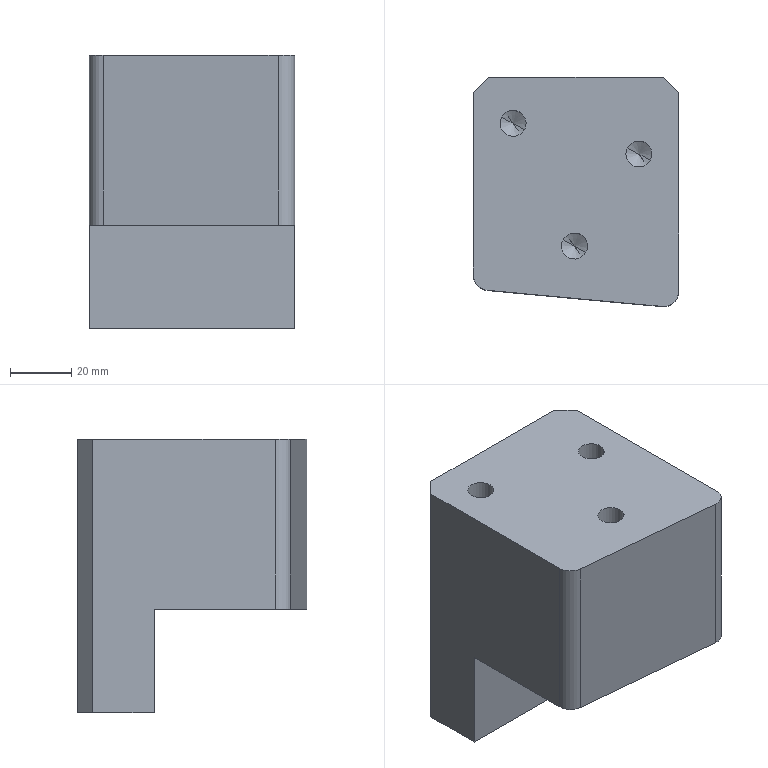Part | CATIA | 1 solid | 40 faces | box 67 x 74.702 x 89 mm | volume 308137 mm3 | cylinder 16 | cone 14 | plane 10 | commonest cylinder face diameters 8.5 x12 10 x4
STEP:
#1=CARTESIAN_POINT('',(81.,85.,84.));
#2=VERTEX_POINT('',#1);
#3=CARTESIAN_POINT('',(86.,90.,84.));
#4=VERTEX_POINT('',#3);
#5=CARTESIAN_POINT('',(83.5,87.5,84.));
#6=DIRECTION('',(-0.7071,-0.7071,0.));
#7=VECTOR('',#6,1.);
#8=LINE('',#5,#7);
#9=EDGE_CURVE('',#2,#4,#8,.F.);
#10=ORIENTED_EDGE('',*,*,#9,.T.);
#11=CARTESIAN_POINT('',(86.,90.,-5.));
#12=VERTEX_POINT('',#11);
#13=CARTESIAN_POINT('',(86.,90.,39.5));
#14=DIRECTION('',(0.,0.,-1.));
#15=VECTOR('',#14,1.);
#16=LINE('',#13,#15);
#17=EDGE_CURVE('',#12,#4,#16,.F.);
#18=ORIENTED_EDGE('',*,*,#17,.F.);
#19=CARTESIAN_POINT('',(81.,85.,-5.));
#20=VERTEX_POINT('',#19);
#21=CARTESIAN_POINT('',(83.5,87.5,-5.));
#22=DIRECTION('',(-0.7071,-0.7071,0.));
#23=VECTOR('',#22,1.);
#24=LINE('',#21,#23);
#25=EDGE_CURVE('',#12,#20,#24,.T.);
#26=ORIENTED_EDGE('',*,*,#25,.T.);
#27=CARTESIAN_POINT('',(81.,85.,39.5));
#28=DIRECTION('',(0.,0.,-1.));
#29=VECTOR('',#28,1.);
#30=LINE('',#27,#29);
#31=EDGE_CURVE('',#20,#2,#30,.F.);
#32=ORIENTED_EDGE('',*,*,#31,.T.);
#33=EDGE_LOOP('',(#10,#18,#26,#32));
#34=FACE_OUTER_BOUND('',#33,.T.);
#35=CARTESIAN_POINT('',(86.,90.,101.8));
#36=DIRECTION('',(-0.7071,0.7071,0.));
#37=DIRECTION('',(0.,0.,-1.));
#38=AXIS2_PLACEMENT_3D('',#35,#36,#37);
#39=PLANE('',#38);
#40=ADVANCED_FACE('',(#34),#39,.T.);
#41=CARTESIAN_POINT('',(143.,90.,-5.));
#42=VERTEX_POINT('',#41);
#43=CARTESIAN_POINT('',(143.,90.,84.));
#44=VERTEX_POINT('',#43);
#45=CARTESIAN_POINT('',(143.,90.,39.5));
#46=DIRECTION('',(0.,0.,1.));
#47=VECTOR('',#46,1.);
#48=LINE('',#45,#47);
#49=EDGE_CURVE('',#42,#44,#48,.T.);
#50=ORIENTED_EDGE('',*,*,#49,.F.);
#51=CARTESIAN_POINT('',(114.5,90.,-5.));
#52=DIRECTION('',(1.,0.,0.));
#53=VECTOR('',#52,1.);
#54=LINE('',#51,#53);
#55=EDGE_CURVE('',#12,#42,#54,.T.);
#56=ORIENTED_EDGE('',*,*,#55,.F.);
#57=ORIENTED_EDGE('',*,*,#17,.T.);
#58=CARTESIAN_POINT('',(114.5,90.,84.));
#59=DIRECTION('',(1.,0.,0.));
#60=VECTOR('',#59,1.);
#61=LINE('',#58,#60);
#62=EDGE_CURVE('',#4,#44,#61,.T.);
#63=ORIENTED_EDGE('',*,*,#62,.T.);
#64=EDGE_LOOP('',(#50,#56,#57,#63));
#65=FACE_OUTER_BOUND('',#64,.T.);
#66=CARTESIAN_POINT('',(81.,90.,0.));
#67=DIRECTION('',(0.,-1.,0.));
#68=DIRECTION('',(1.,0.,0.));
#69=AXIS2_PLACEMENT_3D('',#66,#67,#68);
#70=PLANE('',#69);
#71=ADVANCED_FACE('',(#65),#70,.F.);
#72=CARTESIAN_POINT('',(148.,85.,84.));
#73=VERTEX_POINT('',#72);
#74=CARTESIAN_POINT('',(145.5,87.5,84.));
#75=DIRECTION('',(0.7071,-0.7071,0.));
#76=VECTOR('',#75,1.);
#77=LINE('',#74,#76);
#78=EDGE_CURVE('',#44,#73,#77,.T.);
#79=ORIENTED_EDGE('',*,*,#78,.T.);
#80=CARTESIAN_POINT('',(148.,85.,-5.));
#81=VERTEX_POINT('',#80);
#82=CARTESIAN_POINT('',(148.,85.,39.5));
#83=DIRECTION('',(0.,0.,1.));
#84=VECTOR('',#83,1.);
#85=LINE('',#82,#84);
#86=EDGE_CURVE('',#81,#73,#85,.T.);
#87=ORIENTED_EDGE('',*,*,#86,.F.);
#88=CARTESIAN_POINT('',(145.5,87.5,-5.));
#89=DIRECTION('',(0.7071,-0.7071,0.));
#90=VECTOR('',#89,1.);
#91=LINE('',#88,#90);
#92=EDGE_CURVE('',#81,#42,#91,.F.);
#93=ORIENTED_EDGE('',*,*,#92,.T.);
#94=ORIENTED_EDGE('',*,*,#49,.T.);
#95=EDGE_LOOP('',(#79,#87,#93,#94));
#96=FACE_OUTER_BOUND('',#95,.T.);
#97=CARTESIAN_POINT('',(143.,90.,-22.8));
#98=DIRECTION('',(0.7071,0.7071,0.));
#99=DIRECTION('',(0.,0.,1.));
#100=AXIS2_PLACEMENT_3D('',#97,#98,#99);
#101=PLANE('',#100);
#102=ADVANCED_FACE('',(#96),#101,.T.);
#103=CARTESIAN_POINT('',(114.,35.,51.546));
#104=VERTEX_POINT('',#103);
#105=CARTESIAN_POINT('',(110.27,37.038,54.));
#106=VERTEX_POINT('',#105);
#107=CARTESIAN_POINT('',(112.135,36.019,52.773));
#108=DIRECTION('',(-0.76,0.4152,0.5));
#109=VECTOR('',#108,1.);
#110=LINE('',#107,#109);
#111=EDGE_CURVE('',#104,#106,#110,.T.);
#112=ORIENTED_EDGE('',*,*,#111,.T.);
#113=CARTESIAN_POINT('',(117.73,32.962,54.));
#114=VERTEX_POINT('',#113);
#115=CARTESIAN_POINT('',(114.,35.,54.));
#116=DIRECTION('',(0.,0.,1.));
#117=AXIS2_PLACEMENT_3D('',#115,#116,$);
#118=CIRCLE('',#117,4.25);
#119=EDGE_CURVE('',#114,#106,#118,.F.);
#120=ORIENTED_EDGE('',*,*,#119,.F.);
#121=CARTESIAN_POINT('',(115.865,33.981,52.773));
#122=DIRECTION('',(0.76,-0.4152,0.5));
#123=VECTOR('',#122,1.);
#124=LINE('',#121,#123);
#125=EDGE_CURVE('',#104,#114,#124,.T.);
#126=ORIENTED_EDGE('',*,*,#125,.F.);
#127=EDGE_LOOP('',(#112,#120,#126));
#128=FACE_OUTER_BOUND('',#127,.T.);
#129=CARTESIAN_POINT('',(114.,35.,51.546));
#130=DIRECTION('',(0.,0.,1.));
#131=DIRECTION('',(0.8776,-0.4794,0.));
#132=AXIS2_PLACEMENT_3D('',#129,#130,#131);
#133=CONICAL_SURFACE('',#132,0.,1.047);
#134=ADVANCED_FACE('',(#128),#133,.F.);
#135=ORIENTED_EDGE('',*,*,#125,.T.);
#136=CARTESIAN_POINT('',(114.,35.,54.));
#137=DIRECTION('',(0.,0.,1.));
#138=AXIS2_PLACEMENT_3D('',#136,#137,$);
#139=CIRCLE('',#138,4.25);
#140=EDGE_CURVE('',#106,#114,#139,.F.);
#141=ORIENTED_EDGE('',*,*,#140,.F.);
#142=ORIENTED_EDGE('',*,*,#111,.F.);
#143=EDGE_LOOP('',(#135,#141,#142));
#144=FACE_OUTER_BOUND('',#143,.T.);
#145=ADVANCED_FACE('',(#144),#133,.F.);
#146=CARTESIAN_POINT('',(110.27,37.038,84.));
#147=VERTEX_POINT('',#146);
#148=CARTESIAN_POINT('',(117.73,32.962,84.));
#149=VERTEX_POINT('',#148);
#150=CARTESIAN_POINT('',(114.,35.,84.));
#151=DIRECTION('',(0.,0.,-1.));
#152=AXIS2_PLACEMENT_3D('',#150,#151,$);
#153=CIRCLE('',#152,4.25);
#154=EDGE_CURVE('',#147,#149,#153,.F.);
#155=ORIENTED_EDGE('',*,*,#154,.T.);
#156=CARTESIAN_POINT('',(117.73,32.962,69.2));
#157=DIRECTION('',(0.,0.,-1.));
#158=VECTOR('',#157,1.);
#159=LINE('',#156,#158);
#160=EDGE_CURVE('',#114,#149,#159,.F.);
#161=ORIENTED_EDGE('',*,*,#160,.F.);
#162=ORIENTED_EDGE('',*,*,#119,.T.);
#163=CARTESIAN_POINT('',(110.27,37.038,69.2));
#164=DIRECTION('',(0.,0.,-1.));
#165=VECTOR('',#164,1.);
#166=LINE('',#163,#165);
#167=EDGE_CURVE('',#106,#147,#166,.F.);
#168=ORIENTED_EDGE('',*,*,#167,.T.);
#169=EDGE_LOOP('',(#155,#161,#162,#168));
#170=FACE_OUTER_BOUND('',#169,.T.);
#171=CARTESIAN_POINT('',(114.,35.,83.9));
#172=DIRECTION('',(0.,0.,-1.));
#173=DIRECTION('',(0.8776,-0.4794,0.));
#174=AXIS2_PLACEMENT_3D('',#171,#172,#173);
#175=CYLINDRICAL_SURFACE('',#174,4.25);
#176=ADVANCED_FACE('',(#170),#175,.F.);
#177=CARTESIAN_POINT('',(114.,35.,84.));
#178=DIRECTION('',(0.,0.,-1.));
#179=AXIS2_PLACEMENT_3D('',#177,#178,$);
#180=CIRCLE('',#179,4.25);
#181=EDGE_CURVE('',#149,#147,#180,.F.);
#182=ORIENTED_EDGE('',*,*,#181,.T.);
#183=ORIENTED_EDGE('',*,*,#167,.F.);
#184=ORIENTED_EDGE('',*,*,#140,.T.);
#185=ORIENTED_EDGE('',*,*,#160,.T.);
#186=EDGE_LOOP('',(#182,#183,#184,#185));
#187=FACE_OUTER_BOUND('',#186,.T.);
#188=ADVANCED_FACE('',(#187),#175,.F.);
#189=CARTESIAN_POINT('',(94.,75.,51.546));
#190=VERTEX_POINT('',#189);
#191=CARTESIAN_POINT('',(90.27,77.038,54.));
#192=VERTEX_POINT('',#191);
#193=CARTESIAN_POINT('',(92.135,76.019,52.773));
#194=DIRECTION('',(-0.76,0.4152,0.5));
#195=VECTOR('',#194,1.);
#196=LINE('',#193,#195);
#197=EDGE_CURVE('',#190,#192,#196,.T.);
#198=ORIENTED_EDGE('',*,*,#197,.T.);
#199=CARTESIAN_POINT('',(97.73,72.962,54.));
#200=VERTEX_POINT('',#199);
#201=CARTESIAN_POINT('',(94.,75.,54.));
#202=DIRECTION('',(0.,0.,1.));
#203=AXIS2_PLACEMENT_3D('',#201,#202,$);
#204=CIRCLE('',#203,4.25);
#205=EDGE_CURVE('',#200,#192,#204,.F.);
#206=ORIENTED_EDGE('',*,*,#205,.F.);
#207=CARTESIAN_POINT('',(95.865,73.981,52.773));
#208=DIRECTION('',(0.76,-0.4152,0.5));
#209=VECTOR('',#208,1.);
#210=LINE('',#207,#209);
#211=EDGE_CURVE('',#190,#200,#210,.T.);
#212=ORIENTED_EDGE('',*,*,#211,.F.);
#213=EDGE_LOOP('',(#198,#206,#212));
#214=FACE_OUTER_BOUND('',#213,.T.);
#215=CARTESIAN_POINT('',(94.,75.,51.546));
#216=DIRECTION('',(0.,0.,1.));
#217=DIRECTION('',(0.8776,-0.4794,0.));
#218=AXIS2_PLACEMENT_3D('',#215,#216,#217);
#219=CONICAL_SURFACE('',#218,0.,1.047);
#220=ADVANCED_FACE('',(#214),#219,.F.);
#221=ORIENTED_EDGE('',*,*,#211,.T.);
#222=CARTESIAN_POINT('',(94.,75.,54.));
#223=DIRECTION('',(0.,0.,1.));
#224=AXIS2_PLACEMENT_3D('',#222,#223,$);
#225=CIRCLE('',#224,4.25);
#226=EDGE_CURVE('',#192,#200,#225,.F.);
#227=ORIENTED_EDGE('',*,*,#226,.F.);
#228=ORIENTED_EDGE('',*,*,#197,.F.);
#229=EDGE_LOOP('',(#221,#227,#228));
#230=FACE_OUTER_BOUND('',#229,.T.);
#231=ADVANCED_FACE('',(#230),#219,.F.);
#232=CARTESIAN_POINT('',(90.27,77.038,84.));
#233=VERTEX_POINT('',#232);
#234=CARTESIAN_POINT('',(97.73,72.962,84.));
#235=VERTEX_POINT('',#234);
#236=CARTESIAN_POINT('',(94.,75.,84.));
#237=DIRECTION('',(0.,0.,-1.));
#238=AXIS2_PLACEMENT_3D('',#236,#237,$);
#239=CIRCLE('',#238,4.25);
#240=EDGE_CURVE('',#233,#235,#239,.F.);
#241=ORIENTED_EDGE('',*,*,#240,.T.);
#242=CARTESIAN_POINT('',(97.73,72.962,69.2));
#243=DIRECTION('',(0.,0.,-1.));
#244=VECTOR('',#243,1.);
#245=LINE('',#242,#244);
#246=EDGE_CURVE('',#200,#235,#245,.F.);
#247=ORIENTED_EDGE('',*,*,#246,.F.);
#248=ORIENTED_EDGE('',*,*,#205,.T.);
#249=CARTESIAN_POINT('',(90.27,77.038,69.2));
#250=DIRECTION('',(0.,0.,-1.));
#251=VECTOR('',#250,1.);
#252=LINE('',#249,#251);
#253=EDGE_CURVE('',#192,#233,#252,.F.);
#254=ORIENTED_EDGE('',*,*,#253,.T.);
#255=EDGE_LOOP('',(#241,#247,#248,#254));
#256=FACE_OUTER_BOUND('',#255,.T.);
#257=CARTESIAN_POINT('',(94.,75.,83.9));
#258=DIRECTION('',(0.,0.,-1.));
#259=DIRECTION('',(0.8776,-0.4794,0.));
#260=AXIS2_PLACEMENT_3D('',#257,#258,#259);
#261=CYLINDRICAL_SURFACE('',#260,4.25);
#262=ADVANCED_FACE('',(#256),#261,.F.);
#263=CARTESIAN_POINT('',(94.,75.,84.));
#264=DIRECTION('',(0.,0.,-1.));
#265=AXIS2_PLACEMENT_3D('',#263,#264,$);
#266=CIRCLE('',#265,4.25);
#267=EDGE_CURVE('',#235,#233,#266,.F.);
#268=ORIENTED_EDGE('',*,*,#267,.T.);
#269=ORIENTED_EDGE('',*,*,#253,.F.);
#270=ORIENTED_EDGE('',*,*,#226,.T.);
#271=ORIENTED_EDGE('',*,*,#246,.T.);
#272=EDGE_LOOP('',(#268,#269,#270,#271));
#273=FACE_OUTER_BOUND('',#272,.T.);
#274=ADVANCED_FACE('',(#273),#261,.F.);
#275=CARTESIAN_POINT('',(135.,65.,51.546));
#276=VERTEX_POINT('',#275);
#277=CARTESIAN_POINT('',(131.27,67.038,54.));
#278=VERTEX_POINT('',#277);
#279=CARTESIAN_POINT('',(133.135,66.019,52.773));
#280=DIRECTION('',(-0.76,0.4152,0.5));
#281=VECTOR('',#280,1.);
#282=LINE('',#279,#281);
#283=EDGE_CURVE('',#276,#278,#282,.T.);
#284=ORIENTED_EDGE('',*,*,#283,.T.);
#285=CARTESIAN_POINT('',(138.73,62.962,54.));
#286=VERTEX_POINT('',#285);
#287=CARTESIAN_POINT('',(135.,65.,54.));
#288=DIRECTION('',(0.,0.,1.));
#289=AXIS2_PLACEMENT_3D('',#287,#288,$);
#290=CIRCLE('',#289,4.25);
#291=EDGE_CURVE('',#286,#278,#290,.F.);
#292=ORIENTED_EDGE('',*,*,#291,.F.);
#293=CARTESIAN_POINT('',(136.865,63.981,52.773));
#294=DIRECTION('',(0.76,-0.4152,0.5));
#295=VECTOR('',#294,1.);
#296=LINE('',#293,#295);
#297=EDGE_CURVE('',#276,#286,#296,.T.);
#298=ORIENTED_EDGE('',*,*,#297,.F.);
#299=EDGE_LOOP('',(#284,#292,#298));
#300=FACE_OUTER_BOUND('',#299,.T.);
#301=CARTESIAN_POINT('',(135.,65.,51.546));
#302=DIRECTION('',(0.,0.,1.));
#303=DIRECTION('',(0.8776,-0.4794,0.));
#304=AXIS2_PLACEMENT_3D('',#301,#302,#303);
#305=CONICAL_SURFACE('',#304,0.,1.047);
#306=ADVANCED_FACE('',(#300),#305,.F.);
#307=ORIENTED_EDGE('',*,*,#297,.T.);
#308=CARTESIAN_POINT('',(135.,65.,54.));
#309=DIRECTION('',(0.,0.,1.));
#310=AXIS2_PLACEMENT_3D('',#308,#309,$);
#311=CIRCLE('',#310,4.25);
#312=EDGE_CURVE('',#278,#286,#311,.F.);
#313=ORIENTED_EDGE('',*,*,#312,.F.);
#314=ORIENTED_EDGE('',*,*,#283,.F.);
#315=EDGE_LOOP('',(#307,#313,#314));
#316=FACE_OUTER_BOUND('',#315,.T.);
#317=ADVANCED_FACE('',(#316),#305,.F.);
#318=CARTESIAN_POINT('',(131.27,67.038,84.));
#319=VERTEX_POINT('',#318);
#320=CARTESIAN_POINT('',(138.73,62.962,84.));
#321=VERTEX_POINT('',#320);
#322=CARTESIAN_POINT('',(135.,65.,84.));
#323=DIRECTION('',(0.,0.,-1.));
#324=AXIS2_PLACEMENT_3D('',#322,#323,$);
#325=CIRCLE('',#324,4.25);
#326=EDGE_CURVE('',#319,#321,#325,.F.);
#327=ORIENTED_EDGE('',*,*,#326,.T.);
#328=CARTESIAN_POINT('',(138.73,62.962,69.2));
#329=DIRECTION('',(0.,0.,-1.));
#330=VECTOR('',#329,1.);
#331=LINE('',#328,#330);
#332=EDGE_CURVE('',#286,#321,#331,.F.);
#333=ORIENTED_EDGE('',*,*,#332,.F.);
#334=ORIENTED_EDGE('',*,*,#291,.T.);
#335=CARTESIAN_POINT('',(131.27,67.038,69.2));
#336=DIRECTION('',(0.,0.,-1.));
#337=VECTOR('',#336,1.);
#338=LINE('',#335,#337);
#339=EDGE_CURVE('',#278,#319,#338,.F.);
#340=ORIENTED_EDGE('',*,*,#339,.T.);
#341=EDGE_LOOP('',(#327,#333,#334,#340));
#342=FACE_OUTER_BOUND('',#341,.T.);
#343=CARTESIAN_POINT('',(135.,65.,83.9));
#344=DIRECTION('',(0.,0.,-1.));
#345=DIRECTION('',(0.8776,-0.4794,0.));
#346=AXIS2_PLACEMENT_3D('',#343,#344,#345);
#347=CYLINDRICAL_SURFACE('',#346,4.25);
#348=ADVANCED_FACE('',(#342),#347,.F.);
#349=CARTESIAN_POINT('',(135.,65.,84.));
#350=DIRECTION('',(0.,0.,-1.));
#351=AXIS2_PLACEMENT_3D('',#349,#350,$);
#352=CIRCLE('',#351,4.25);
#353=EDGE_CURVE('',#321,#319,#352,.F.);
#354=ORIENTED_EDGE('',*,*,#353,.T.);
#355=ORIENTED_EDGE('',*,*,#339,.F.);
#356=ORIENTED_EDGE('',*,*,#312,.T.);
#357=ORIENTED_EDGE('',*,*,#332,.T.);
#358=EDGE_LOOP('',(#354,#355,#356,#357));
#359=FACE_OUTER_BOUND('',#358,.T.);
#360=ADVANCED_FACE('',(#359),#347,.F.);
#361=CARTESIAN_POINT('',(94.,52.,61.454));
#362=VERTEX_POINT('',#361);
#363=CARTESIAN_POINT('',(90.27,49.962,59.));
#364=VERTEX_POINT('',#363);
#365=CARTESIAN_POINT('',(92.135,50.981,60.227));
#366=DIRECTION('',(-0.76,-0.4152,-0.5));
#367=VECTOR('',#366,1.);
#368=LINE('',#365,#367);
#369=EDGE_CURVE('',#362,#364,#368,.T.);
#370=ORIENTED_EDGE('',*,*,#369,.T.);
#371=CARTESIAN_POINT('',(97.73,54.038,59.));
#372=VERTEX_POINT('',#371);
#373=CARTESIAN_POINT('',(94.,52.,59.));
#374=DIRECTION('',(0.,0.,-1.));
#375=AXIS2_PLACEMENT_3D('',#373,#374,$);
#376=CIRCLE('',#375,4.25);
#377=EDGE_CURVE('',#372,#364,#376,.F.);
#378=ORIENTED_EDGE('',*,*,#377,.F.);
#379=CARTESIAN_POINT('',(95.865,53.019,60.227));
#380=DIRECTION('',(0.76,0.4152,-0.5));
#381=VECTOR('',#380,1.);
#382=LINE('',#379,#381);
#383=EDGE_CURVE('',#362,#372,#382,.T.);
#384=ORIENTED_EDGE('',*,*,#383,.F.);
#385=EDGE_LOOP('',(#370,#378,#384));
#386=FACE_OUTER_BOUND('',#385,.T.);
#387=CARTESIAN_POINT('',(94.,52.,61.454));
#388=DIRECTION('',(0.,0.,-1.));
#389=DIRECTION('',(0.8776,0.4794,0.));
#390=AXIS2_PLACEMENT_3D('',#387,#388,#389);
#391=CONICAL_SURFACE('',#390,0.,1.047);
#392=ADVANCED_FACE('',(#386),#391,.F.);
#393=ORIENTED_EDGE('',*,*,#383,.T.);
#394=CARTESIAN_POINT('',(94.,52.,59.));
#395=DIRECTION('',(0.,0.,-1.));
#396=AXIS2_PLACEMENT_3D('',#394,#395,$);
#397=CIRCLE('',#396,4.25);
#398=EDGE_CURVE('',#364,#372,#397,.F.);
#399=ORIENTED_EDGE('',*,*,#398,.F.);
#400=ORIENTED_EDGE('',*,*,#369,.F.);
#401=EDGE_LOOP('',(#393,#399,#400));
#402=FACE_OUTER_BOUND('',#401,.T.);
#403=ADVANCED_FACE('',(#402),#391,.F.);
#404=CARTESIAN_POINT('',(97.73,54.038,28.7));
#405=VERTEX_POINT('',#404);
#406=CARTESIAN_POINT('',(90.27,49.962,28.7));
#407=VERTEX_POINT('',#406);
#408=CARTESIAN_POINT('',(94.,52.,28.7));
#409=DIRECTION('',(0.,0.,1.));
#410=AXIS2_PLACEMENT_3D('',#408,#409,$);
#411=CIRCLE('',#410,4.25);
#412=EDGE_CURVE('',#405,#407,#411,.T.);
#413=ORIENTED_EDGE('',*,*,#412,.F.);
#414=CARTESIAN_POINT('',(97.73,54.038,41.345));
#415=DIRECTION('',(0.,0.,1.));
#416=VECTOR('',#415,1.);
#417=LINE('',#414,#416);
#418=EDGE_CURVE('',#372,#405,#417,.F.);
#419=ORIENTED_EDGE('',*,*,#418,.F.);
#420=ORIENTED_EDGE('',*,*,#377,.T.);
#421=CARTESIAN_POINT('',(90.27,49.962,41.345));
#422=DIRECTION('',(0.,0.,1.));
#423=VECTOR('',#422,1.);
#424=LINE('',#421,#423);
#425=EDGE_CURVE('',#364,#407,#424,.F.);
#426=ORIENTED_EDGE('',*,*,#425,.T.);
#427=EDGE_LOOP('',(#413,#419,#420,#426));
#428=FACE_OUTER_BOUND('',#427,.T.);
#429=CARTESIAN_POINT('',(94.,52.,24.1));
#430=DIRECTION('',(0.,0.,1.));
#431=DIRECTION('',(0.8776,0.4794,0.));
#432=AXIS2_PLACEMENT_3D('',#429,#430,#431);
#433=CYLINDRICAL_SURFACE('',#432,4.25);
#434=ADVANCED_FACE('',(#428),#433,.F.);
#435=CARTESIAN_POINT('',(94.,52.,28.7));
#436=DIRECTION('',(0.,0.,1.));
#437=AXIS2_PLACEMENT_3D('',#435,#436,$);
#438=CIRCLE('',#437,4.25);
#439=EDGE_CURVE('',#407,#405,#438,.T.);
#440=ORIENTED_EDGE('',*,*,#439,.F.);
#441=ORIENTED_EDGE('',*,*,#425,.F.);
#442=ORIENTED_EDGE('',*,*,#398,.T.);
#443=ORIENTED_EDGE('',*,*,#418,.T.);
#444=EDGE_LOOP('',(#440,#441,#442,#443));
#445=FACE_OUTER_BOUND('',#444,.T.);
#446=ADVANCED_FACE('',(#445),#433,.F.);
#447=CARTESIAN_POINT('',(81.,65.,28.7));
#448=VERTEX_POINT('',#447);
#449=CARTESIAN_POINT('',(81.,65.,-5.));
#450=VERTEX_POINT('',#449);
#451=CARTESIAN_POINT('',(81.,65.,11.85));
#452=DIRECTION('',(0.,0.,-1.));
#453=VECTOR('',#452,1.);
#454=LINE('',#451,#453);
#455=EDGE_CURVE('',#448,#450,#454,.T.);
#456=ORIENTED_EDGE('',*,*,#455,.T.);
#457=CARTESIAN_POINT('',(148.,65.,-5.));
#458=VERTEX_POINT('',#457);
#459=CARTESIAN_POINT('',(114.5,65.,-5.));
#460=DIRECTION('',(1.,0.,0.));
#461=VECTOR('',#460,1.);
#462=LINE('',#459,#461);
#463=EDGE_CURVE('',#450,#458,#462,.T.);
#464=ORIENTED_EDGE('',*,*,#463,.T.);
#465=CARTESIAN_POINT('',(148.,65.,28.7));
#466=VERTEX_POINT('',#465);
#467=CARTESIAN_POINT('',(148.,65.,11.85));
#468=DIRECTION('',(0.,0.,-1.));
#469=VECTOR('',#468,1.);
#470=LINE('',#467,#469);
#471=EDGE_CURVE('',#466,#458,#470,.T.);
#472=ORIENTED_EDGE('',*,*,#471,.F.);
#473=CARTESIAN_POINT('',(114.5,65.,28.7));
#474=DIRECTION('',(1.,0.,0.));
#475=VECTOR('',#474,1.);
#476=LINE('',#473,#475);
#477=EDGE_CURVE('',#466,#448,#476,.F.);
#478=ORIENTED_EDGE('',*,*,#477,.T.);
#479=EDGE_LOOP('',(#456,#464,#472,#478));
#480=FACE_OUTER_BOUND('',#479,.T.);
#481=CARTESIAN_POINT('',(74.,65.,24.));
#482=DIRECTION('',(0.,1.,0.));
#483=DIRECTION('',(1.,0.,0.));
#484=AXIS2_PLACEMENT_3D('',#481,#482,#483);
#485=PLANE('',#484);
#486=ADVANCED_FACE('',(#480),#485,.F.);
#487=CARTESIAN_POINT('',(138.73,54.038,28.7));
#488=VERTEX_POINT('',#487);
#489=CARTESIAN_POINT('',(131.27,49.962,28.7));
#490=VERTEX_POINT('',#489);
#491=CARTESIAN_POINT('',(135.,52.,28.7));
#492=DIRECTION('',(0.,0.,1.));
#493=AXIS2_PLACEMENT_3D('',#491,#492,$);
#494=CIRCLE('',#493,4.25);
#495=EDGE_CURVE('',#488,#490,#494,.T.);
#496=ORIENTED_EDGE('',*,*,#495,.F.);
#497=CARTESIAN_POINT('',(138.73,54.038,59.));
#498=VERTEX_POINT('',#497);
#499=CARTESIAN_POINT('',(138.73,54.038,41.345));
#500=DIRECTION('',(0.,0.,1.));
#501=VECTOR('',#500,1.);
#502=LINE('',#499,#501);
#503=EDGE_CURVE('',#498,#488,#502,.F.);
#504=ORIENTED_EDGE('',*,*,#503,.F.);
#505=CARTESIAN_POINT('',(131.27,49.962,59.));
#506=VERTEX_POINT('',#505);
#507=CARTESIAN_POINT('',(135.,52.,59.));
#508=DIRECTION('',(0.,0.,1.));
#509=AXIS2_PLACEMENT_3D('',#507,#508,$);
#510=CIRCLE('',#509,4.25);
#511=EDGE_CURVE('',#498,#506,#510,.T.);
#512=ORIENTED_EDGE('',*,*,#511,.T.);
#513=CARTESIAN_POINT('',(131.27,49.962,41.345));
#514=DIRECTION('',(0.,0.,1.));
#515=VECTOR('',#514,1.);
#516=LINE('',#513,#515);
#517=EDGE_CURVE('',#506,#490,#516,.F.);
#518=ORIENTED_EDGE('',*,*,#517,.T.);
#519=EDGE_LOOP('',(#496,#504,#512,#518));
#520=FACE_OUTER_BOUND('',#519,.T.);
#521=CARTESIAN_POINT('',(135.,52.,24.1));
#522=DIRECTION('',(0.,0.,1.));
#523=DIRECTION('',(0.8776,0.4794,0.));
#524=AXIS2_PLACEMENT_3D('',#521,#522,#523);
#525=CYLINDRICAL_SURFACE('',#524,4.25);
#526=ADVANCED_FACE('',(#520),#525,.F.);
#527=CARTESIAN_POINT('',(135.,52.,28.7));
#528=DIRECTION('',(0.,0.,1.));
#529=AXIS2_PLACEMENT_3D('',#527,#528,$);
#530=CIRCLE('',#529,4.25);
#531=EDGE_CURVE('',#490,#488,#530,.T.);
#532=ORIENTED_EDGE('',*,*,#531,.F.);
#533=ORIENTED_EDGE('',*,*,#517,.F.);
#534=CARTESIAN_POINT('',(135.,52.,59.));
#535=DIRECTION('',(0.,0.,1.));
#536=AXIS2_PLACEMENT_3D('',#534,#535,$);
#537=CIRCLE('',#536,4.25);
#538=EDGE_CURVE('',#506,#498,#537,.T.);
#539=ORIENTED_EDGE('',*,*,#538,.T.);
#540=ORIENTED_EDGE('',*,*,#503,.T.);
#541=EDGE_LOOP('',(#532,#533,#539,#540));
#542=FACE_OUTER_BOUND('',#541,.T.);
#543=ADVANCED_FACE('',(#542),#525,.F.);
#544=CARTESIAN_POINT('',(117.388,54.397,28.7));
#545=VERTEX_POINT('',#544);
#546=CARTESIAN_POINT('',(108.612,49.603,28.7));
#547=VERTEX_POINT('',#546);
#548=CARTESIAN_POINT('',(113.,52.,28.7));
#549=DIRECTION('',(0.,0.,1.));
#550=AXIS2_PLACEMENT_3D('',#548,#549,$);
#551=CIRCLE('',#550,5.);
#552=EDGE_CURVE('',#545,#547,#551,.T.);
#553=ORIENTED_EDGE('',*,*,#552,.F.);
#554=CARTESIAN_POINT('',(117.388,54.397,54.));
#555=VERTEX_POINT('',#554);
#556=CARTESIAN_POINT('',(117.388,54.397,38.845));
#557=DIRECTION('',(0.,0.,1.));
#558=VECTOR('',#557,1.);
#559=LINE('',#556,#558);
#560=EDGE_CURVE('',#555,#545,#559,.F.);
#561=ORIENTED_EDGE('',*,*,#560,.F.);
#562=CARTESIAN_POINT('',(108.612,49.603,54.));
#563=VERTEX_POINT('',#562);
#564=CARTESIAN_POINT('',(113.,52.,54.));
#565=DIRECTION('',(0.,0.,1.));
#566=AXIS2_PLACEMENT_3D('',#564,#565,$);
#567=CIRCLE('',#566,5.);
#568=EDGE_CURVE('',#555,#563,#567,.T.);
#569=ORIENTED_EDGE('',*,*,#568,.T.);
#570=CARTESIAN_POINT('',(108.612,49.603,38.845));
#571=DIRECTION('',(0.,0.,1.));
#572=VECTOR('',#571,1.);
#573=LINE('',#570,#572);
#574=EDGE_CURVE('',#563,#547,#573,.F.);
#575=ORIENTED_EDGE('',*,*,#574,.T.);
#576=EDGE_LOOP('',(#553,#561,#569,#575));
#577=FACE_OUTER_BOUND('',#576,.T.);
#578=CARTESIAN_POINT('',(113.,52.,24.1));
#579=DIRECTION('',(0.,0.,1.));
#580=DIRECTION('',(0.8776,0.4794,0.));
#581=AXIS2_PLACEMENT_3D('',#578,#579,#580);
#582=CYLINDRICAL_SURFACE('',#581,5.);
#583=ADVANCED_FACE('',(#577),#582,.F.);
#584=CARTESIAN_POINT('',(113.,52.,28.7));
#585=DIRECTION('',(0.,0.,1.));
#586=AXIS2_PLACEMENT_3D('',#584,#585,$);
#587=CIRCLE('',#586,5.);
#588=EDGE_CURVE('',#547,#545,#587,.T.);
#589=ORIENTED_EDGE('',*,*,#588,.F.);
#590=ORIENTED_EDGE('',*,*,#574,.F.);
#591=CARTESIAN_POINT('',(113.,52.,54.));
#592=DIRECTION('',(0.,0.,1.));
#593=AXIS2_PLACEMENT_3D('',#591,#592,$);
#594=CIRCLE('',#593,5.);
#595=EDGE_CURVE('',#563,#555,#594,.T.);
#596=ORIENTED_EDGE('',*,*,#595,.T.);
#597=ORIENTED_EDGE('',*,*,#560,.T.);
#598=EDGE_LOOP('',(#589,#590,#596,#597));
#599=FACE_OUTER_BOUND('',#598,.T.);
#600=ADVANCED_FACE('',(#599),#582,.F.);
#601=CARTESIAN_POINT('',(135.,52.,61.454));
#602=VERTEX_POINT('',#601);
#603=CARTESIAN_POINT('',(133.135,50.981,60.227));
#604=DIRECTION('',(-0.76,-0.4152,-0.5));
#605=VECTOR('',#604,1.);
#606=LINE('',#603,#605);
#607=EDGE_CURVE('',#602,#506,#606,.T.);
#608=ORIENTED_EDGE('',*,*,#607,.T.);
#609=ORIENTED_EDGE('',*,*,#511,.F.);
#610=CARTESIAN_POINT('',(136.865,53.019,60.227));
#611=DIRECTION('',(0.76,0.4152,-0.5));
#612=VECTOR('',#611,1.);
#613=LINE('',#610,#612);
#614=EDGE_CURVE('',#602,#498,#613,.T.);
#615=ORIENTED_EDGE('',*,*,#614,.F.);
#616=EDGE_LOOP('',(#608,#609,#615));
#617=FACE_OUTER_BOUND('',#616,.T.);
#618=CARTESIAN_POINT('',(135.,52.,61.454));
#619=DIRECTION('',(0.,0.,-1.));
#620=DIRECTION('',(0.8776,0.4794,0.));
#621=AXIS2_PLACEMENT_3D('',#618,#619,#620);
#622=CONICAL_SURFACE('',#621,0.,1.047);
#623=ADVANCED_FACE('',(#617),#622,.F.);
#624=ORIENTED_EDGE('',*,*,#614,.T.);
#625=ORIENTED_EDGE('',*,*,#538,.F.);
#626=ORIENTED_EDGE('',*,*,#607,.F.);
#627=EDGE_LOOP('',(#624,#625,#626));
#628=FACE_OUTER_BOUND('',#627,.T.);
#629=ADVANCED_FACE('',(#628),#622,.F.);
#630=CARTESIAN_POINT('',(113.,52.,56.887));
#631=VERTEX_POINT('',#630);
#632=CARTESIAN_POINT('',(110.806,50.801,55.443));
#633=DIRECTION('',(-0.76,-0.4152,-0.5));
#634=VECTOR('',#633,1.);
#635=LINE('',#632,#634);
#636=EDGE_CURVE('',#631,#563,#635,.T.);
#637=ORIENTED_EDGE('',*,*,#636,.T.);
#638=ORIENTED_EDGE('',*,*,#568,.F.);
#639=CARTESIAN_POINT('',(115.194,53.199,55.443));
#640=DIRECTION('',(0.76,0.4152,-0.5));
#641=VECTOR('',#640,1.);
#642=LINE('',#639,#641);
#643=EDGE_CURVE('',#631,#555,#642,.T.);
#644=ORIENTED_EDGE('',*,*,#643,.F.);
#645=EDGE_LOOP('',(#637,#638,#644));
#646=FACE_OUTER_BOUND('',#645,.T.);
#647=CARTESIAN_POINT('',(113.,52.,56.887));
#648=DIRECTION('',(0.,0.,-1.));
#649=DIRECTION('',(0.8776,0.4794,0.));
#650=AXIS2_PLACEMENT_3D('',#647,#648,#649);
#651=CONICAL_SURFACE('',#650,0.,1.047);
#652=ADVANCED_FACE('',(#646),#651,.F.);
#653=ORIENTED_EDGE('',*,*,#643,.T.);
#654=ORIENTED_EDGE('',*,*,#595,.F.);
#655=ORIENTED_EDGE('',*,*,#636,.F.);
#656=EDGE_LOOP('',(#653,#654,#655));
#657=FACE_OUTER_BOUND('',#656,.T.);
#658=ADVANCED_FACE('',(#657),#651,.F.);
#659=CARTESIAN_POINT('',(81.,75.,-5.));
#660=DIRECTION('',(0.,-1.,0.));
#661=VECTOR('',#660,1.);
#662=LINE('',#659,#661);
#663=EDGE_CURVE('',#450,#20,#662,.F.);
#664=ORIENTED_EDGE('',*,*,#663,.T.);
#665=ORIENTED_EDGE('',*,*,#25,.F.);
#666=ORIENTED_EDGE('',*,*,#55,.T.);
#667=ORIENTED_EDGE('',*,*,#92,.F.);
#668=CARTESIAN_POINT('',(148.,75.,-5.));
#669=DIRECTION('',(0.,1.,0.));
#670=VECTOR('',#669,1.);
#671=LINE('',#668,#670);
#672=EDGE_CURVE('',#81,#458,#671,.F.);
#673=ORIENTED_EDGE('',*,*,#672,.T.);
#674=ORIENTED_EDGE('',*,*,#463,.F.);
#675=EDGE_LOOP('',(#664,#665,#666,#667,#673,#674));
#676=FACE_OUTER_BOUND('',#675,.T.);
#677=CARTESIAN_POINT('',(118.73,79.038,-5.));
#678=VERTEX_POINT('',#677);
#679=CARTESIAN_POINT('',(111.27,74.962,-5.));
#680=VERTEX_POINT('',#679);
#681=CARTESIAN_POINT('',(115.,77.,-5.));
#682=DIRECTION('',(0.,0.,-1.));
#683=AXIS2_PLACEMENT_3D('',#681,#682,$);
#684=CIRCLE('',#683,4.25);
#685=EDGE_CURVE('',#678,#680,#684,.T.);
#686=ORIENTED_EDGE('',*,*,#685,.F.);
#687=CARTESIAN_POINT('',(115.,77.,-5.));
#688=DIRECTION('',(0.,0.,-1.));
#689=AXIS2_PLACEMENT_3D('',#687,#688,$);
#690=CIRCLE('',#689,4.25);
#691=EDGE_CURVE('',#680,#678,#690,.T.);
#692=ORIENTED_EDGE('',*,*,#691,.F.);
#693=EDGE_LOOP('',(#686,#692));
#694=FACE_BOUND('',#693,.T.);
#695=CARTESIAN_POINT('',(0.,0.,-5.));
#696=DIRECTION('',(0.,0.,-1.));
#697=DIRECTION('',(1.,0.,0.));
#698=AXIS2_PLACEMENT_3D('',#695,#696,#697);
#699=PLANE('',#698);
#700=ADVANCED_FACE('',(#676,#694),#699,.T.);
#701=CARTESIAN_POINT('',(115.,77.,27.454));
#702=VERTEX_POINT('',#701);
#703=CARTESIAN_POINT('',(111.27,74.962,25.));
#704=VERTEX_POINT('',#703);
#705=CARTESIAN_POINT('',(113.135,75.981,26.227));
#706=DIRECTION('',(-0.76,-0.4152,-0.5));
#707=VECTOR('',#706,1.);
#708=LINE('',#705,#707);
#709=EDGE_CURVE('',#702,#704,#708,.T.);
#710=ORIENTED_EDGE('',*,*,#709,.T.);
#711=CARTESIAN_POINT('',(118.73,79.038,25.));
#712=VERTEX_POINT('',#711);
#713=CARTESIAN_POINT('',(115.,77.,25.));
#714=DIRECTION('',(0.,0.,-1.));
#715=AXIS2_PLACEMENT_3D('',#713,#714,$);
#716=CIRCLE('',#715,4.25);
#717=EDGE_CURVE('',#712,#704,#716,.F.);
#718=ORIENTED_EDGE('',*,*,#717,.F.);
#719=CARTESIAN_POINT('',(116.865,78.019,26.227));
#720=DIRECTION('',(0.76,0.4152,-0.5));
#721=VECTOR('',#720,1.);
#722=LINE('',#719,#721);
#723=EDGE_CURVE('',#702,#712,#722,.T.);
#724=ORIENTED_EDGE('',*,*,#723,.F.);
#725=EDGE_LOOP('',(#710,#718,#724));
#726=FACE_OUTER_BOUND('',#725,.T.);
#727=CARTESIAN_POINT('',(115.,77.,27.454));
#728=DIRECTION('',(0.,0.,-1.));
#729=DIRECTION('',(0.8776,0.4794,0.));
#730=AXIS2_PLACEMENT_3D('',#727,#728,#729);
#731=CONICAL_SURFACE('',#730,0.,1.047);
#732=ADVANCED_FACE('',(#726),#731,.F.);
#733=ORIENTED_EDGE('',*,*,#723,.T.);
#734=CARTESIAN_POINT('',(115.,77.,25.));
#735=DIRECTION('',(0.,0.,-1.));
#736=AXIS2_PLACEMENT_3D('',#734,#735,$);
#737=CIRCLE('',#736,4.25);
#738=EDGE_CURVE('',#704,#712,#737,.F.);
#739=ORIENTED_EDGE('',*,*,#738,.F.);
#740=ORIENTED_EDGE('',*,*,#709,.F.);
#741=EDGE_LOOP('',(#733,#739,#740));
#742=FACE_OUTER_BOUND('',#741,.T.);
#743=ADVANCED_FACE('',(#742),#731,.F.);
#744=ORIENTED_EDGE('',*,*,#691,.T.);
#745=CARTESIAN_POINT('',(118.73,79.038,9.8));
#746=DIRECTION('',(0.,0.,1.));
#747=VECTOR('',#746,1.);
#748=LINE('',#745,#747);
#749=EDGE_CURVE('',#712,#678,#748,.F.);
#750=ORIENTED_EDGE('',*,*,#749,.F.);
#751=ORIENTED_EDGE('',*,*,#717,.T.);
#752=CARTESIAN_POINT('',(111.27,74.962,9.8));
#753=DIRECTION('',(0.,0.,1.));
#754=VECTOR('',#753,1.);
#755=LINE('',#752,#754);
#756=EDGE_CURVE('',#704,#680,#755,.F.);
#757=ORIENTED_EDGE('',*,*,#756,.T.);
#758=EDGE_LOOP('',(#744,#750,#751,#757));
#759=FACE_OUTER_BOUND('',#758,.T.);
#760=CARTESIAN_POINT('',(115.,77.,-4.9));
#761=DIRECTION('',(0.,0.,1.));
#762=DIRECTION('',(0.8776,0.4794,0.));
#763=AXIS2_PLACEMENT_3D('',#760,#761,#762);
#764=CYLINDRICAL_SURFACE('',#763,4.25);
#765=ADVANCED_FACE('',(#759),#764,.F.);
#766=ORIENTED_EDGE('',*,*,#685,.T.);
#767=ORIENTED_EDGE('',*,*,#756,.F.);
#768=ORIENTED_EDGE('',*,*,#738,.T.);
#769=ORIENTED_EDGE('',*,*,#749,.T.);
#770=EDGE_LOOP('',(#766,#767,#768,#769));
#771=FACE_OUTER_BOUND('',#770,.T.);
#772=ADVANCED_FACE('',(#771),#764,.F.);
#773=CARTESIAN_POINT('',(148.,20.298,28.7));
#774=VERTEX_POINT('',#773);
#775=CARTESIAN_POINT('',(148.,42.649,28.7));
#776=DIRECTION('',(0.,-1.,0.));
#777=VECTOR('',#776,1.);
#778=LINE('',#775,#777);
#779=EDGE_CURVE('',#466,#774,#778,.T.);
#780=ORIENTED_EDGE('',*,*,#779,.F.);
#781=ORIENTED_EDGE('',*,*,#471,.T.);
#782=ORIENTED_EDGE('',*,*,#672,.F.);
#783=ORIENTED_EDGE('',*,*,#86,.T.);
#784=CARTESIAN_POINT('',(148.,20.298,84.));
#785=VERTEX_POINT('',#784);
#786=CARTESIAN_POINT('',(148.,52.649,84.));
#787=DIRECTION('',(0.,1.,0.));
#788=VECTOR('',#787,1.);
#789=LINE('',#786,#788);
#790=EDGE_CURVE('',#785,#73,#789,.T.);
#791=ORIENTED_EDGE('',*,*,#790,.F.);
#792=CARTESIAN_POINT('',(148.,20.298,56.35));
#793=DIRECTION('',(0.,0.,-1.));
#794=VECTOR('',#793,1.);
#795=LINE('',#792,#794);
#796=EDGE_CURVE('',#774,#785,#795,.F.);
#797=ORIENTED_EDGE('',*,*,#796,.F.);
#798=EDGE_LOOP('',(#780,#781,#782,#783,#791,#797));
#799=FACE_OUTER_BOUND('',#798,.T.);
#800=CARTESIAN_POINT('',(148.,15.,0.));
#801=DIRECTION('',(1.,0.,0.));
#802=DIRECTION('',(0.,1.,0.));
#803=AXIS2_PLACEMENT_3D('',#800,#801,#802);
#804=PLANE('',#803);
#805=ADVANCED_FACE('',(#799),#804,.T.);
#806=CARTESIAN_POINT('',(142.54,15.319,84.));
#807=VERTEX_POINT('',#806);
#808=CARTESIAN_POINT('',(143.,20.298,84.));
#809=DIRECTION('',(0.,0.,-1.));
#810=AXIS2_PLACEMENT_3D('',#808,#809,$);
#811=CIRCLE('',#810,5.);
#812=EDGE_CURVE('',#785,#807,#811,.T.);
#813=ORIENTED_EDGE('',*,*,#812,.T.);
#814=CARTESIAN_POINT('',(142.54,15.319,28.7));
#815=VERTEX_POINT('',#814);
#816=CARTESIAN_POINT('',(142.54,15.319,39.5));
#817=DIRECTION('',(0.,0.,-1.));
#818=VECTOR('',#817,1.);
#819=LINE('',#816,#818);
#820=EDGE_CURVE('',#815,#807,#819,.F.);
#821=ORIENTED_EDGE('',*,*,#820,.F.);
#822=CARTESIAN_POINT('',(143.,20.298,28.7));
#823=DIRECTION('',(0.,0.,-1.));
#824=AXIS2_PLACEMENT_3D('',#822,#823,$);
#825=CIRCLE('',#824,5.);
#826=EDGE_CURVE('',#815,#774,#825,.F.);
#827=ORIENTED_EDGE('',*,*,#826,.T.);
#828=ORIENTED_EDGE('',*,*,#796,.T.);
#829=EDGE_LOOP('',(#813,#821,#827,#828));
#830=FACE_OUTER_BOUND('',#829,.T.);
#831=CARTESIAN_POINT('',(143.,20.298,39.5));
#832=DIRECTION('',(0.,0.,-1.));
#833=DIRECTION('',(1.,0.,0.));
#834=AXIS2_PLACEMENT_3D('',#831,#832,#833);
#835=CYLINDRICAL_SURFACE('',#834,5.);
#836=ADVANCED_FACE('',(#830),#835,.T.);
#837=CARTESIAN_POINT('',(81.,25.56,84.));
#838=VERTEX_POINT('',#837);
#839=CARTESIAN_POINT('',(81.,55.28,84.));
#840=DIRECTION('',(0.,-1.,0.));
#841=VECTOR('',#840,1.);
#842=LINE('',#839,#841);
#843=EDGE_CURVE('',#2,#838,#842,.T.);
#844=ORIENTED_EDGE('',*,*,#843,.F.);
#845=ORIENTED_EDGE('',*,*,#31,.F.);
#846=ORIENTED_EDGE('',*,*,#663,.F.);
#847=ORIENTED_EDGE('',*,*,#455,.F.);
#848=CARTESIAN_POINT('',(81.,25.56,28.7));
#849=VERTEX_POINT('',#848);
#850=CARTESIAN_POINT('',(81.,45.28,28.7));
#851=DIRECTION('',(0.,-1.,0.));
#852=VECTOR('',#851,1.);
#853=LINE('',#850,#852);
#854=EDGE_CURVE('',#448,#849,#853,.T.);
#855=ORIENTED_EDGE('',*,*,#854,.T.);
#856=CARTESIAN_POINT('',(81.,25.56,56.35));
#857=DIRECTION('',(0.,0.,-1.));
#858=VECTOR('',#857,1.);
#859=LINE('',#856,#858);
#860=EDGE_CURVE('',#849,#838,#859,.F.);
#861=ORIENTED_EDGE('',*,*,#860,.T.);
#862=EDGE_LOOP('',(#844,#845,#846,#847,#855,#861));
#863=FACE_OUTER_BOUND('',#862,.T.);
#864=CARTESIAN_POINT('',(81.,90.,0.));
#865=DIRECTION('',(-1.,0.,0.));
#866=DIRECTION('',(0.,-1.,0.));
#867=AXIS2_PLACEMENT_3D('',#864,#865,#866);
#868=PLANE('',#867);
#869=ADVANCED_FACE('',(#863),#868,.T.);
#870=CARTESIAN_POINT('',(85.54,20.581,28.7));
#871=VERTEX_POINT('',#870);
#872=CARTESIAN_POINT('',(113.5,18.,28.7));
#873=DIRECTION('',(0.9958,-0.09192,0.));
#874=VECTOR('',#873,1.);
#875=LINE('',#872,#874);
#876=EDGE_CURVE('',#871,#815,#875,.T.);
#877=ORIENTED_EDGE('',*,*,#876,.T.);
#878=ORIENTED_EDGE('',*,*,#820,.T.);
#879=CARTESIAN_POINT('',(85.54,20.581,84.));
#880=VERTEX_POINT('',#879);
#881=CARTESIAN_POINT('',(113.5,18.,84.));
#882=DIRECTION('',(0.9958,-0.09192,0.));
#883=VECTOR('',#882,1.);
#884=LINE('',#881,#883);
#885=EDGE_CURVE('',#807,#880,#884,.F.);
#886=ORIENTED_EDGE('',*,*,#885,.T.);
#887=CARTESIAN_POINT('',(85.54,20.581,39.5));
#888=DIRECTION('',(0.,0.,-1.));
#889=VECTOR('',#888,1.);
#890=LINE('',#887,#889);
#891=EDGE_CURVE('',#871,#880,#890,.F.);
#892=ORIENTED_EDGE('',*,*,#891,.F.);
#893=EDGE_LOOP('',(#877,#878,#886,#892));
#894=FACE_OUTER_BOUND('',#893,.T.);
#895=CARTESIAN_POINT('',(81.,21.,101.8));
#896=DIRECTION('',(-0.09192,-0.9958,0.));
#897=DIRECTION('',(0.,0.,-1.));
#898=AXIS2_PLACEMENT_3D('',#895,#896,#897);
#899=PLANE('',#898);
#900=ADVANCED_FACE('',(#894),#899,.T.);
#901=ORIENTED_EDGE('',*,*,#885,.F.);
#902=ORIENTED_EDGE('',*,*,#812,.F.);
#903=ORIENTED_EDGE('',*,*,#790,.T.);
#904=ORIENTED_EDGE('',*,*,#78,.F.);
#905=ORIENTED_EDGE('',*,*,#62,.F.);
#906=ORIENTED_EDGE('',*,*,#9,.F.);
#907=ORIENTED_EDGE('',*,*,#843,.T.);
#908=CARTESIAN_POINT('',(86.,25.56,84.));
#909=DIRECTION('',(0.,0.,1.));
#910=AXIS2_PLACEMENT_3D('',#908,#909,$);
#911=CIRCLE('',#910,5.);
#912=EDGE_CURVE('',#880,#838,#911,.F.);
#913=ORIENTED_EDGE('',*,*,#912,.F.);
#914=EDGE_LOOP('',(#901,#902,#903,#904,#905,#906,#907,#913));
#915=FACE_OUTER_BOUND('',#914,.T.);
#916=ORIENTED_EDGE('',*,*,#353,.F.);
#917=ORIENTED_EDGE('',*,*,#326,.F.);
#918=EDGE_LOOP('',(#916,#917));
#919=FACE_BOUND('',#918,.T.);
#920=ORIENTED_EDGE('',*,*,#267,.F.);
#921=ORIENTED_EDGE('',*,*,#240,.F.);
#922=EDGE_LOOP('',(#920,#921));
#923=FACE_BOUND('',#922,.T.);
#924=ORIENTED_EDGE('',*,*,#181,.F.);
#925=ORIENTED_EDGE('',*,*,#154,.F.);
#926=EDGE_LOOP('',(#924,#925));
#927=FACE_BOUND('',#926,.T.);
#928=CARTESIAN_POINT('',(0.,0.,84.));
#929=DIRECTION('',(0.,0.,1.));
#930=DIRECTION('',(1.,0.,0.));
#931=AXIS2_PLACEMENT_3D('',#928,#929,#930);
#932=PLANE('',#931);
#933=ADVANCED_FACE('',(#915,#919,#923,#927),#932,.T.);
#934=CARTESIAN_POINT('',(86.,25.56,28.7));
#935=DIRECTION('',(0.,0.,1.));
#936=AXIS2_PLACEMENT_3D('',#934,#935,$);
#937=CIRCLE('',#936,5.);
#938=EDGE_CURVE('',#849,#871,#937,.T.);
#939=ORIENTED_EDGE('',*,*,#938,.F.);
#940=ORIENTED_EDGE('',*,*,#854,.F.);
#941=ORIENTED_EDGE('',*,*,#477,.F.);
#942=ORIENTED_EDGE('',*,*,#779,.T.);
#943=ORIENTED_EDGE('',*,*,#826,.F.);
#944=ORIENTED_EDGE('',*,*,#876,.F.);
#945=EDGE_LOOP('',(#939,#940,#941,#942,#943,#944));
#946=FACE_OUTER_BOUND('',#945,.T.);
#947=ORIENTED_EDGE('',*,*,#439,.T.);
#948=ORIENTED_EDGE('',*,*,#412,.T.);
#949=EDGE_LOOP('',(#947,#948));
#950=FACE_BOUND('',#949,.T.);
#951=ORIENTED_EDGE('',*,*,#531,.T.);
#952=ORIENTED_EDGE('',*,*,#495,.T.);
#953=EDGE_LOOP('',(#951,#952));
#954=FACE_BOUND('',#953,.T.);
#955=ORIENTED_EDGE('',*,*,#588,.T.);
#956=ORIENTED_EDGE('',*,*,#552,.T.);
#957=EDGE_LOOP('',(#955,#956));
#958=FACE_BOUND('',#957,.T.);
#959=CARTESIAN_POINT('',(0.,0.,28.7));
#960=DIRECTION('',(0.,0.,1.));
#961=DIRECTION('',(1.,0.,0.));
#962=AXIS2_PLACEMENT_3D('',#959,#960,#961);
#963=PLANE('',#962);
#964=ADVANCED_FACE('',(#946,#950,#954,#958),#963,.F.);
#965=ORIENTED_EDGE('',*,*,#912,.T.);
#966=ORIENTED_EDGE('',*,*,#860,.F.);
#967=ORIENTED_EDGE('',*,*,#938,.T.);
#968=ORIENTED_EDGE('',*,*,#891,.T.);
#969=EDGE_LOOP('',(#965,#966,#967,#968));
#970=FACE_OUTER_BOUND('',#969,.T.);
#971=CARTESIAN_POINT('',(86.,25.56,39.5));
#972=DIRECTION('',(0.,0.,-1.));
#973=DIRECTION('',(-0.09192,-0.9958,0.));
#974=AXIS2_PLACEMENT_3D('',#971,#972,#973);
#975=CYLINDRICAL_SURFACE('',#974,5.);
#976=ADVANCED_FACE('',(#970),#975,.T.);
#977=CLOSED_SHELL('',(#40,#71,#102,#134,#145,#176,#188,#220,#231,#262,#274,#306,#317,#348,#360,#392,#403,#434,#446,#486,#526,#543,#583,#600,#623,#629,#652,#658,#700,#732,#743,#765,#772,#805,#836,#869,#900,#933,#964,#976));
#978=MANIFOLD_SOLID_BREP('',#977);
#979=(LENGTH_UNIT()NAMED_UNIT(*)SI_UNIT(.MILLI.,.METRE.));
#980=UNCERTAINTY_MEASURE_WITH_UNIT(LENGTH_MEASURE(0.005),#979,'','');
#981=(NAMED_UNIT(*)PLANE_ANGLE_UNIT()SI_UNIT($,.RADIAN.));
#982=(NAMED_UNIT(*)SI_UNIT($,.STERADIAN.)SOLID_ANGLE_UNIT());
#983=(GEOMETRIC_REPRESENTATION_CONTEXT(3)GLOBAL_UNCERTAINTY_ASSIGNED_CONTEXT((#980))GLOBAL_UNIT_ASSIGNED_CONTEXT((#979,#981,#982))REPRESENTATION_CONTEXT('',''));
#984=ADVANCED_BREP_SHAPE_REPRESENTATION('',(#978),#983);